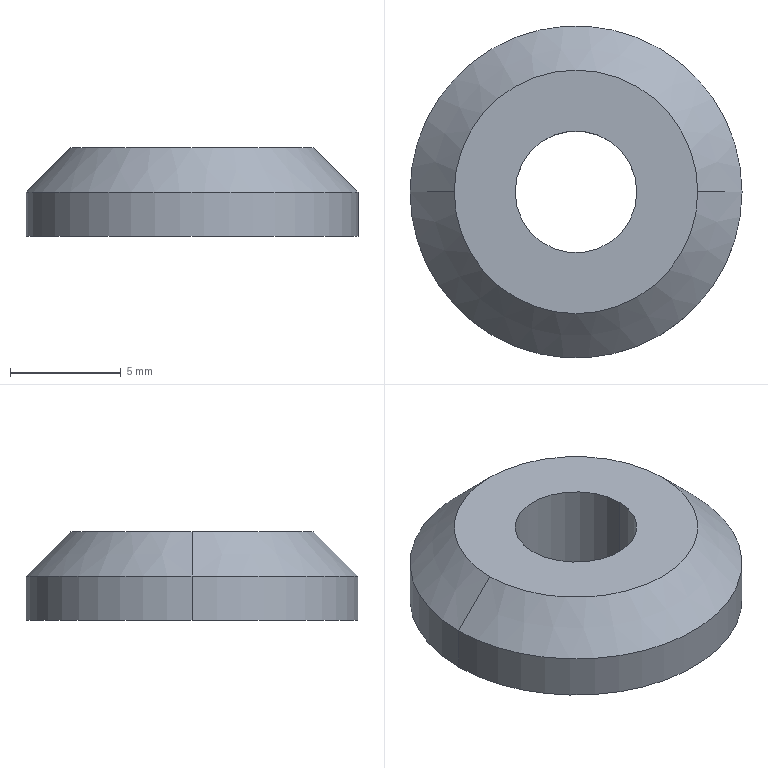Part | NX | features BREP 1 | 1 solid | 8 faces | box 15 x 15 x 4 mm | volume 525.955 mm3 | cylinder 4 | cone 2 | plane 2 | commonest cylinder face diameters 5.5 x2 15 x2
STEP:
#1=CARTESIAN_POINT('',(236.798,-120.614,0.));
#2=VERTEX_POINT('',#1);
#3=CARTESIAN_POINT('',(242.298,-120.614,0.));
#4=VERTEX_POINT('',#3);
#5=CARTESIAN_POINT('',(239.548,-120.614,0.));
#6=DIRECTION('',(0.,0.,1.));
#7=DIRECTION('',(1.,0.,0.));
#8=AXIS2_PLACEMENT_3D('',#5,#6,#7);
#9=CIRCLE('',#8,2.75);
#10=EDGE_CURVE('',#2,#4,#9,.T.);
#11=ORIENTED_EDGE('',*,*,#10,.F.);
#12=CARTESIAN_POINT('',(236.798,-120.614,4.));
#13=VERTEX_POINT('',#12);
#14=CARTESIAN_POINT('',(236.798,-120.614,0.));
#15=DIRECTION('',(0.,0.,1.));
#16=VECTOR('',#15,1000.);
#17=LINE('',#14,#16);
#18=EDGE_CURVE('',#13,#2,#17,.F.);
#19=ORIENTED_EDGE('',*,*,#18,.F.);
#20=CARTESIAN_POINT('',(242.298,-120.614,4.));
#21=VERTEX_POINT('',#20);
#22=CARTESIAN_POINT('',(239.548,-120.614,4.));
#23=DIRECTION('',(0.,0.,1.));
#24=DIRECTION('',(1.,0.,0.));
#25=AXIS2_PLACEMENT_3D('',#22,#23,#24);
#26=CIRCLE('',#25,2.75);
#27=EDGE_CURVE('',#13,#21,#26,.T.);
#28=ORIENTED_EDGE('',*,*,#27,.T.);
#29=CARTESIAN_POINT('',(242.298,-120.614,0.));
#30=DIRECTION('',(0.,0.,1.));
#31=VECTOR('',#30,1000.);
#32=LINE('',#29,#31);
#33=EDGE_CURVE('',#21,#4,#32,.F.);
#34=ORIENTED_EDGE('',*,*,#33,.T.);
#35=EDGE_LOOP('',(#11,#19,#28,#34));
#36=FACE_BOUND('',#35,.T.);
#37=CARTESIAN_POINT('',(239.548,-120.614,0.));
#38=DIRECTION('',(0.,0.,1.));
#39=DIRECTION('',(1.,0.,0.));
#40=AXIS2_PLACEMENT_3D('',#37,#38,#39);
#41=CYLINDRICAL_SURFACE('',#40,2.75);
#42=ADVANCED_FACE('',(#36),#41,.F.);
#43=CARTESIAN_POINT('',(245.048,-120.614,4.));
#44=VERTEX_POINT('',#43);
#45=CARTESIAN_POINT('',(234.048,-120.614,4.));
#46=VERTEX_POINT('',#45);
#47=CARTESIAN_POINT('',(239.548,-120.614,4.));
#48=DIRECTION('',(0.,0.,1.));
#49=DIRECTION('',(1.,0.,0.));
#50=AXIS2_PLACEMENT_3D('',#47,#48,#49);
#51=CIRCLE('',#50,5.5);
#52=EDGE_CURVE('',#44,#46,#51,.T.);
#53=ORIENTED_EDGE('',*,*,#52,.F.);
#54=CARTESIAN_POINT('',(247.048,-120.614,2.));
#55=VERTEX_POINT('',#54);
#56=CARTESIAN_POINT('',(245.048,-120.614,4.));
#57=DIRECTION('',(0.7071,0.,-0.7071));
#58=VECTOR('',#57,1000.);
#59=LINE('',#56,#58);
#60=EDGE_CURVE('',#44,#55,#59,.T.);
#61=ORIENTED_EDGE('',*,*,#60,.T.);
#62=CARTESIAN_POINT('',(232.048,-120.614,2.));
#63=VERTEX_POINT('',#62);
#64=CARTESIAN_POINT('',(239.548,-120.614,2.));
#65=DIRECTION('',(0.,0.,-1.));
#66=DIRECTION('',(1.,0.,0.));
#67=AXIS2_PLACEMENT_3D('',#64,#65,#66);
#68=CIRCLE('',#67,7.5);
#69=EDGE_CURVE('',#63,#55,#68,.T.);
#70=ORIENTED_EDGE('',*,*,#69,.F.);
#71=CARTESIAN_POINT('',(234.048,-120.614,4.));
#72=DIRECTION('',(-0.7071,0.,-0.7071));
#73=VECTOR('',#72,1000.);
#74=LINE('',#71,#73);
#75=EDGE_CURVE('',#46,#63,#74,.T.);
#76=ORIENTED_EDGE('',*,*,#75,.F.);
#77=EDGE_LOOP('',(#53,#61,#70,#76));
#78=FACE_BOUND('',#77,.T.);
#79=CARTESIAN_POINT('',(239.548,-120.614,4.));
#80=DIRECTION('',(0.,0.,-1.));
#81=DIRECTION('',(-1.,0.,0.));
#82=AXIS2_PLACEMENT_3D('',#79,#80,#81);
#83=CONICAL_SURFACE('',#82,5.5,0.7854);
#84=ADVANCED_FACE('',(#78),#83,.T.);
#85=ORIENTED_EDGE('',*,*,#69,.T.);
#86=CARTESIAN_POINT('',(247.048,-120.614,0.));
#87=VERTEX_POINT('',#86);
#88=CARTESIAN_POINT('',(247.048,-120.614,4.));
#89=DIRECTION('',(0.,0.,-1.));
#90=VECTOR('',#89,1000.);
#91=LINE('',#88,#90);
#92=EDGE_CURVE('',#55,#87,#91,.T.);
#93=ORIENTED_EDGE('',*,*,#92,.T.);
#94=CARTESIAN_POINT('',(232.048,-120.614,0.));
#95=VERTEX_POINT('',#94);
#96=CARTESIAN_POINT('',(239.548,-120.614,0.));
#97=DIRECTION('',(0.,0.,1.));
#98=DIRECTION('',(1.,0.,0.));
#99=AXIS2_PLACEMENT_3D('',#96,#97,#98);
#100=CIRCLE('',#99,7.5);
#101=EDGE_CURVE('',#87,#95,#100,.T.);
#102=ORIENTED_EDGE('',*,*,#101,.T.);
#103=CARTESIAN_POINT('',(232.048,-120.614,4.));
#104=DIRECTION('',(0.,0.,-1.));
#105=VECTOR('',#104,1000.);
#106=LINE('',#103,#105);
#107=EDGE_CURVE('',#63,#95,#106,.T.);
#108=ORIENTED_EDGE('',*,*,#107,.F.);
#109=EDGE_LOOP('',(#85,#93,#102,#108));
#110=FACE_BOUND('',#109,.T.);
#111=CARTESIAN_POINT('',(239.548,-120.614,4.));
#112=DIRECTION('',(0.,0.,-1.));
#113=DIRECTION('',(-1.,0.,0.));
#114=AXIS2_PLACEMENT_3D('',#111,#112,#113);
#115=CYLINDRICAL_SURFACE('',#114,7.5);
#116=ADVANCED_FACE('',(#110),#115,.T.);
#117=ORIENTED_EDGE('',*,*,#92,.F.);
#118=CARTESIAN_POINT('',(239.548,-120.614,2.));
#119=DIRECTION('',(0.,0.,-1.));
#120=DIRECTION('',(1.,0.,0.));
#121=AXIS2_PLACEMENT_3D('',#118,#119,#120);
#122=CIRCLE('',#121,7.5);
#123=EDGE_CURVE('',#55,#63,#122,.T.);
#124=ORIENTED_EDGE('',*,*,#123,.T.);
#125=ORIENTED_EDGE('',*,*,#107,.T.);
#126=CARTESIAN_POINT('',(239.548,-120.614,0.));
#127=DIRECTION('',(0.,0.,1.));
#128=DIRECTION('',(1.,0.,0.));
#129=AXIS2_PLACEMENT_3D('',#126,#127,#128);
#130=CIRCLE('',#129,7.5);
#131=EDGE_CURVE('',#95,#87,#130,.T.);
#132=ORIENTED_EDGE('',*,*,#131,.T.);
#133=EDGE_LOOP('',(#117,#124,#125,#132));
#134=FACE_BOUND('',#133,.T.);
#135=CARTESIAN_POINT('',(239.548,-120.614,4.));
#136=DIRECTION('',(0.,0.,-1.));
#137=DIRECTION('',(-1.,0.,0.));
#138=AXIS2_PLACEMENT_3D('',#135,#136,#137);
#139=CYLINDRICAL_SURFACE('',#138,7.5);
#140=ADVANCED_FACE('',(#134),#139,.T.);
#141=CARTESIAN_POINT('',(239.548,-120.614,4.));
#142=DIRECTION('',(0.,0.,1.));
#143=DIRECTION('',(1.,0.,0.));
#144=AXIS2_PLACEMENT_3D('',#141,#142,#143);
#145=CIRCLE('',#144,5.5);
#146=EDGE_CURVE('',#46,#44,#145,.T.);
#147=ORIENTED_EDGE('',*,*,#146,.T.);
#148=ORIENTED_EDGE('',*,*,#52,.T.);
#149=EDGE_LOOP('',(#147,#148));
#150=FACE_BOUND('',#149,.T.);
#151=CARTESIAN_POINT('',(239.548,-120.614,4.));
#152=DIRECTION('',(0.,0.,1.));
#153=DIRECTION('',(1.,0.,0.));
#154=AXIS2_PLACEMENT_3D('',#151,#152,#153);
#155=CIRCLE('',#154,2.75);
#156=EDGE_CURVE('',#21,#13,#155,.T.);
#157=ORIENTED_EDGE('',*,*,#156,.F.);
#158=ORIENTED_EDGE('',*,*,#27,.F.);
#159=EDGE_LOOP('',(#157,#158));
#160=FACE_BOUND('',#159,.T.);
#161=CARTESIAN_POINT('',(239.548,-120.614,4.));
#162=DIRECTION('',(0.,0.,1.));
#163=DIRECTION('',(1.,0.,0.));
#164=AXIS2_PLACEMENT_3D('',#161,#162,#163);
#165=PLANE('',#164);
#166=ADVANCED_FACE('',(#150,#160),#165,.T.);
#167=ORIENTED_EDGE('',*,*,#131,.F.);
#168=ORIENTED_EDGE('',*,*,#101,.F.);
#169=EDGE_LOOP('',(#167,#168));
#170=FACE_BOUND('',#169,.T.);
#171=CARTESIAN_POINT('',(239.548,-120.614,0.));
#172=DIRECTION('',(0.,0.,1.));
#173=DIRECTION('',(1.,0.,0.));
#174=AXIS2_PLACEMENT_3D('',#171,#172,#173);
#175=CIRCLE('',#174,2.75);
#176=EDGE_CURVE('',#4,#2,#175,.T.);
#177=ORIENTED_EDGE('',*,*,#176,.T.);
#178=ORIENTED_EDGE('',*,*,#10,.T.);
#179=EDGE_LOOP('',(#177,#178));
#180=FACE_BOUND('',#179,.T.);
#181=CARTESIAN_POINT('',(239.548,-120.614,0.));
#182=DIRECTION('',(0.,0.,1.));
#183=DIRECTION('',(1.,0.,0.));
#184=AXIS2_PLACEMENT_3D('',#181,#182,#183);
#185=PLANE('',#184);
#186=ADVANCED_FACE('',(#170,#180),#185,.F.);
#187=ORIENTED_EDGE('',*,*,#60,.F.);
#188=ORIENTED_EDGE('',*,*,#146,.F.);
#189=ORIENTED_EDGE('',*,*,#75,.T.);
#190=ORIENTED_EDGE('',*,*,#123,.F.);
#191=EDGE_LOOP('',(#187,#188,#189,#190));
#192=FACE_BOUND('',#191,.T.);
#193=CARTESIAN_POINT('',(239.548,-120.614,4.));
#194=DIRECTION('',(0.,0.,-1.));
#195=DIRECTION('',(-1.,0.,0.));
#196=AXIS2_PLACEMENT_3D('',#193,#194,#195);
#197=CONICAL_SURFACE('',#196,5.5,0.7854);
#198=ADVANCED_FACE('',(#192),#197,.T.);
#199=ORIENTED_EDGE('',*,*,#18,.T.);
#200=ORIENTED_EDGE('',*,*,#176,.F.);
#201=ORIENTED_EDGE('',*,*,#33,.F.);
#202=ORIENTED_EDGE('',*,*,#156,.T.);
#203=EDGE_LOOP('',(#199,#200,#201,#202));
#204=FACE_BOUND('',#203,.T.);
#205=CARTESIAN_POINT('',(239.548,-120.614,0.));
#206=DIRECTION('',(0.,0.,1.));
#207=DIRECTION('',(1.,0.,0.));
#208=AXIS2_PLACEMENT_3D('',#205,#206,#207);
#209=CYLINDRICAL_SURFACE('',#208,2.75);
#210=ADVANCED_FACE('',(#204),#209,.F.);
#211=CLOSED_SHELL('',(#42,#84,#116,#140,#166,#186,#198,#210));
#212=MANIFOLD_SOLID_BREP('',#211);
#213=(LENGTH_UNIT()NAMED_UNIT(*)SI_UNIT(.MILLI.,.METRE.));
#214=UNCERTAINTY_MEASURE_WITH_UNIT(LENGTH_MEASURE(0.00001),#213,'','');
#215=(NAMED_UNIT(*)PLANE_ANGLE_UNIT()SI_UNIT($,.RADIAN.));
#216=(NAMED_UNIT(*)SI_UNIT($,.STERADIAN.)SOLID_ANGLE_UNIT());
#217=(GEOMETRIC_REPRESENTATION_CONTEXT(3)GLOBAL_UNCERTAINTY_ASSIGNED_CONTEXT((#214))GLOBAL_UNIT_ASSIGNED_CONTEXT((#213,#215,#216))REPRESENTATION_CONTEXT('',''));
#218=ADVANCED_BREP_SHAPE_REPRESENTATION('',(#212),#217);